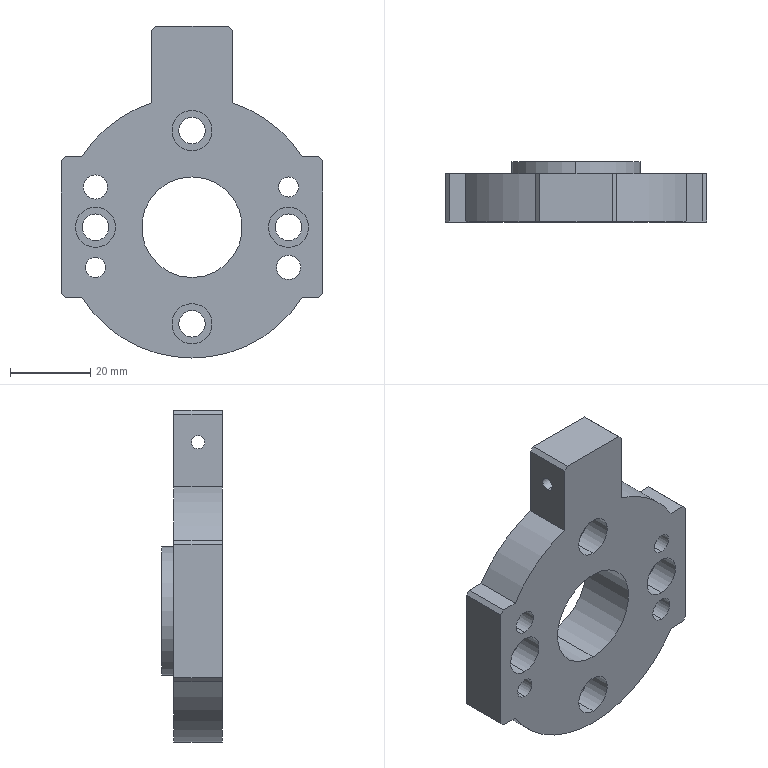Part | SolidWorks | features HoleWzd 4, Cut 2, Chamfer 1, Extrusion 1 | 1 solid | 56 faces | box 65 x 15 x 82.5 mm | volume 36373 mm3 | cylinder 34 | plane 22 | commonest cylinder face diameters 6.6 x8 10 x8 5 x4 6 x4 65 x4 3.3 x2